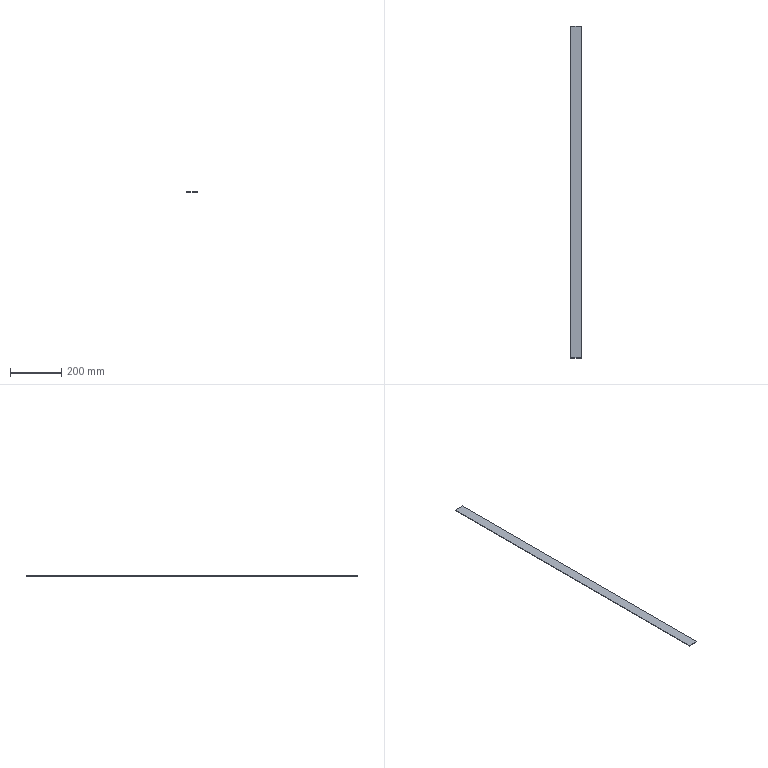Part | NX | features BREP 1 | 1 solid | 6 faces | box 40 x 1300 x 2 mm | volume 104000 mm3 | plane 6
STEP:
#1=CARTESIAN_POINT('',(2024.081,650.,67.));
#2=VERTEX_POINT('',#1);
#3=CARTESIAN_POINT('',(1984.081,650.,67.));
#4=VERTEX_POINT('',#3);
#5=CARTESIAN_POINT('',(2004.081,650.,67.));
#6=DIRECTION('',(-1.,0.,0.));
#7=VECTOR('',#6,1000.);
#8=LINE('',#5,#7);
#9=EDGE_CURVE('',#2,#4,#8,.T.);
#10=ORIENTED_EDGE('',*,*,#9,.F.);
#11=CARTESIAN_POINT('',(2024.081,650.,65.));
#12=VERTEX_POINT('',#11);
#13=CARTESIAN_POINT('',(2024.081,650.,66.));
#14=DIRECTION('',(0.,0.,1.));
#15=VECTOR('',#14,1000.);
#16=LINE('',#13,#15);
#17=EDGE_CURVE('',#12,#2,#16,.T.);
#18=ORIENTED_EDGE('',*,*,#17,.F.);
#19=CARTESIAN_POINT('',(1984.081,650.,65.));
#20=VERTEX_POINT('',#19);
#21=CARTESIAN_POINT('',(2004.081,650.,65.));
#22=DIRECTION('',(-1.,0.,0.));
#23=VECTOR('',#22,1000.);
#24=LINE('',#21,#23);
#25=EDGE_CURVE('',#12,#20,#24,.T.);
#26=ORIENTED_EDGE('',*,*,#25,.T.);
#27=CARTESIAN_POINT('',(1984.081,650.,66.));
#28=DIRECTION('',(0.,0.,1.));
#29=VECTOR('',#28,1000.);
#30=LINE('',#27,#29);
#31=EDGE_CURVE('',#20,#4,#30,.T.);
#32=ORIENTED_EDGE('',*,*,#31,.T.);
#33=EDGE_LOOP('',(#10,#18,#26,#32));
#34=FACE_BOUND('',#33,.T.);
#35=CARTESIAN_POINT('',(2004.081,650.,67.));
#36=DIRECTION('',(0.,-1.,0.));
#37=DIRECTION('',(1.,0.,0.));
#38=AXIS2_PLACEMENT_3D('',#35,#36,#37);
#39=PLANE('',#38);
#40=ADVANCED_FACE('',(#34),#39,.F.);
#41=CARTESIAN_POINT('',(1984.081,-650.,67.));
#42=VERTEX_POINT('',#41);
#43=CARTESIAN_POINT('',(2024.081,-650.,67.));
#44=VERTEX_POINT('',#43);
#45=CARTESIAN_POINT('',(2004.081,-650.,67.));
#46=DIRECTION('',(1.,0.,0.));
#47=VECTOR('',#46,1000.);
#48=LINE('',#45,#47);
#49=EDGE_CURVE('',#42,#44,#48,.T.);
#50=ORIENTED_EDGE('',*,*,#49,.T.);
#51=CARTESIAN_POINT('',(2024.081,0.,67.));
#52=DIRECTION('',(0.,-1.,0.));
#53=VECTOR('',#52,1000.);
#54=LINE('',#51,#53);
#55=EDGE_CURVE('',#2,#44,#54,.T.);
#56=ORIENTED_EDGE('',*,*,#55,.F.);
#57=ORIENTED_EDGE('',*,*,#9,.T.);
#58=CARTESIAN_POINT('',(1984.081,0.,67.));
#59=DIRECTION('',(0.,-1.,0.));
#60=VECTOR('',#59,1000.);
#61=LINE('',#58,#60);
#62=EDGE_CURVE('',#4,#42,#61,.T.);
#63=ORIENTED_EDGE('',*,*,#62,.T.);
#64=EDGE_LOOP('',(#50,#56,#57,#63));
#65=FACE_BOUND('',#64,.T.);
#66=CARTESIAN_POINT('',(836.881,-30.,67.));
#67=DIRECTION('',(0.,0.,-1.));
#68=DIRECTION('',(0.,-1.,0.));
#69=AXIS2_PLACEMENT_3D('',#66,#67,#68);
#70=PLANE('',#69);
#71=ADVANCED_FACE('',(#65),#70,.F.);
#72=CARTESIAN_POINT('',(2024.081,-650.,65.));
#73=VERTEX_POINT('',#72);
#74=CARTESIAN_POINT('',(2024.081,-650.,66.));
#75=DIRECTION('',(0.,0.,1.));
#76=VECTOR('',#75,1000.);
#77=LINE('',#74,#76);
#78=EDGE_CURVE('',#73,#44,#77,.T.);
#79=ORIENTED_EDGE('',*,*,#78,.F.);
#80=CARTESIAN_POINT('',(2024.081,0.000000001,65.));
#81=DIRECTION('',(0.,-1.,0.));
#82=VECTOR('',#81,1000.);
#83=LINE('',#80,#82);
#84=EDGE_CURVE('',#12,#73,#83,.T.);
#85=ORIENTED_EDGE('',*,*,#84,.F.);
#86=ORIENTED_EDGE('',*,*,#17,.T.);
#87=ORIENTED_EDGE('',*,*,#55,.T.);
#88=EDGE_LOOP('',(#79,#85,#86,#87));
#89=FACE_BOUND('',#88,.T.);
#90=CARTESIAN_POINT('',(2024.081,-325.,67.));
#91=DIRECTION('',(1.,0.,0.));
#92=DIRECTION('',(0.,1.,0.));
#93=AXIS2_PLACEMENT_3D('',#90,#91,#92);
#94=PLANE('',#93);
#95=ADVANCED_FACE('',(#89),#94,.T.);
#96=CARTESIAN_POINT('',(1984.081,-650.,65.));
#97=VERTEX_POINT('',#96);
#98=CARTESIAN_POINT('',(1984.081,0.,65.));
#99=DIRECTION('',(0.,-1.,0.));
#100=VECTOR('',#99,1000.);
#101=LINE('',#98,#100);
#102=EDGE_CURVE('',#20,#97,#101,.T.);
#103=ORIENTED_EDGE('',*,*,#102,.F.);
#104=ORIENTED_EDGE('',*,*,#25,.F.);
#105=ORIENTED_EDGE('',*,*,#84,.T.);
#106=CARTESIAN_POINT('',(2004.081,-650.,65.));
#107=DIRECTION('',(1.,0.,0.));
#108=VECTOR('',#107,1000.);
#109=LINE('',#106,#108);
#110=EDGE_CURVE('',#97,#73,#109,.T.);
#111=ORIENTED_EDGE('',*,*,#110,.F.);
#112=EDGE_LOOP('',(#103,#104,#105,#111));
#113=FACE_BOUND('',#112,.T.);
#114=CARTESIAN_POINT('',(836.881,-30.,65.));
#115=DIRECTION('',(0.,0.,-1.));
#116=DIRECTION('',(0.,-1.,0.));
#117=AXIS2_PLACEMENT_3D('',#114,#115,#116);
#118=PLANE('',#117);
#119=ADVANCED_FACE('',(#113),#118,.T.);
#120=ORIENTED_EDGE('',*,*,#62,.F.);
#121=ORIENTED_EDGE('',*,*,#31,.F.);
#122=ORIENTED_EDGE('',*,*,#102,.T.);
#123=CARTESIAN_POINT('',(1984.081,-650.,66.));
#124=DIRECTION('',(0.,0.,1.));
#125=VECTOR('',#124,1000.);
#126=LINE('',#123,#125);
#127=EDGE_CURVE('',#97,#42,#126,.T.);
#128=ORIENTED_EDGE('',*,*,#127,.T.);
#129=EDGE_LOOP('',(#120,#121,#122,#128));
#130=FACE_BOUND('',#129,.T.);
#131=CARTESIAN_POINT('',(1984.081,-325.,67.));
#132=DIRECTION('',(-1.,0.,0.));
#133=DIRECTION('',(0.,1.,0.));
#134=AXIS2_PLACEMENT_3D('',#131,#132,#133);
#135=PLANE('',#134);
#136=ADVANCED_FACE('',(#130),#135,.T.);
#137=ORIENTED_EDGE('',*,*,#127,.F.);
#138=ORIENTED_EDGE('',*,*,#110,.T.);
#139=ORIENTED_EDGE('',*,*,#78,.T.);
#140=ORIENTED_EDGE('',*,*,#49,.F.);
#141=EDGE_LOOP('',(#137,#138,#139,#140));
#142=FACE_BOUND('',#141,.T.);
#143=CARTESIAN_POINT('',(2004.081,-650.,67.));
#144=DIRECTION('',(0.,-1.,0.));
#145=DIRECTION('',(1.,0.,0.));
#146=AXIS2_PLACEMENT_3D('',#143,#144,#145);
#147=PLANE('',#146);
#148=ADVANCED_FACE('',(#142),#147,.T.);
#149=CLOSED_SHELL('',(#40,#71,#95,#119,#136,#148));
#150=MANIFOLD_SOLID_BREP('',#149);
#151=(LENGTH_UNIT()NAMED_UNIT(*)SI_UNIT(.MILLI.,.METRE.));
#152=UNCERTAINTY_MEASURE_WITH_UNIT(LENGTH_MEASURE(0.00001),#151,'','');
#153=(NAMED_UNIT(*)PLANE_ANGLE_UNIT()SI_UNIT($,.RADIAN.));
#154=(NAMED_UNIT(*)SI_UNIT($,.STERADIAN.)SOLID_ANGLE_UNIT());
#155=(GEOMETRIC_REPRESENTATION_CONTEXT(3)GLOBAL_UNCERTAINTY_ASSIGNED_CONTEXT((#152))GLOBAL_UNIT_ASSIGNED_CONTEXT((#151,#153,#154))REPRESENTATION_CONTEXT('',''));
#156=ADVANCED_BREP_SHAPE_REPRESENTATION('',(#150),#155);